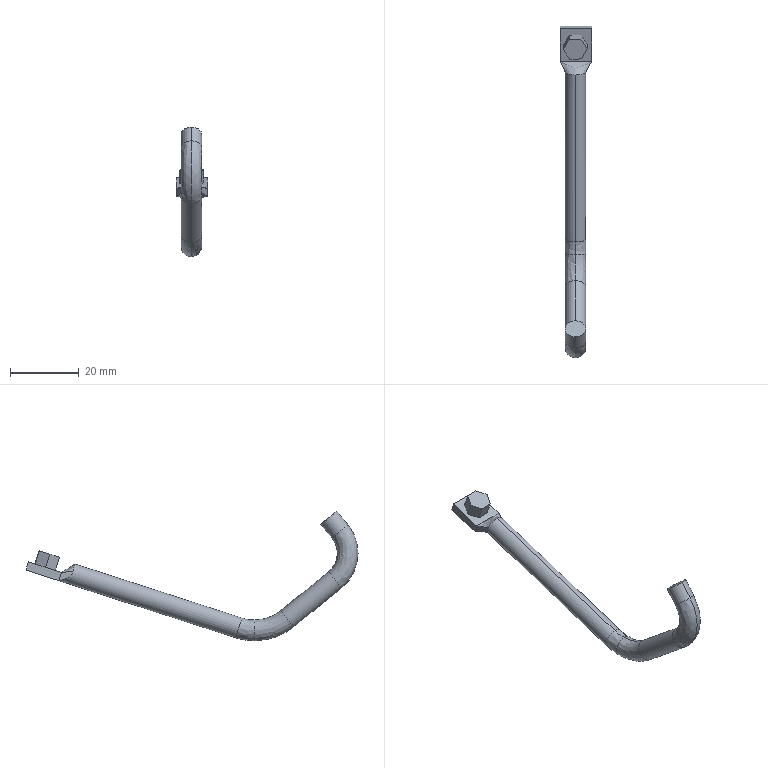Part | SolidWorks | features BaseBody 2 | 2 solids | 30 faces | box 9.082 x 96.3 x 37.547 mm | volume 3383 mm3 | plane 14 | spline 10 | cylinder 6 | commonest cylinder face diameters 6 x6
STEP:
#1=CARTESIAN_POINT('',(0.000000001,-80.618,2441.417));
#2=VERTEX_POINT('',#1);
#3=CARTESIAN_POINT('',(0.000000001,-76.83,2446.069));
#4=VERTEX_POINT('',#3);
#5=CARTESIAN_POINT('',(0.,-78.724,2443.743));
#6=DIRECTION('',(0.,-0.7755,0.6314));
#7=DIRECTION('',(0.,0.6314,0.7755));
#8=AXIS2_PLACEMENT_3D('',#5,#6,#7);
#9=CIRCLE('',#8,3.);
#10=EDGE_CURVE('',#2,#4,#9,.T.);
#11=ORIENTED_EDGE('',*,*,#10,.F.);
#12=CARTESIAN_POINT('',(0.,-66.764,2430.136));
#13=VERTEX_POINT('',#12);
#14=CARTESIAN_POINT('',(0.,-80.618,2441.417));
#15=DIRECTION('',(0.,0.7755,-0.6314));
#16=VECTOR('',#15,1000.);
#17=LINE('',#14,#16);
#18=EDGE_CURVE('',#2,#13,#17,.T.);
#19=ORIENTED_EDGE('',*,*,#18,.T.);
#20=CARTESIAN_POINT('',(0.000000001,-62.975,2434.789));
#21=VERTEX_POINT('',#20);
#22=CARTESIAN_POINT('',(0.,-64.869,2432.462));
#23=DIRECTION('',(0.,0.7755,-0.6314));
#24=DIRECTION('',(0.,0.6314,0.7755));
#25=AXIS2_PLACEMENT_3D('',#22,#23,#24);
#26=CIRCLE('',#25,3.);
#27=EDGE_CURVE('',#21,#13,#26,.T.);
#28=ORIENTED_EDGE('',*,*,#27,.F.);
#29=CARTESIAN_POINT('',(0.,-76.83,2446.069));
#30=DIRECTION('',(0.,0.7755,-0.6314));
#31=VECTOR('',#30,1000.);
#32=LINE('',#29,#31);
#33=EDGE_CURVE('',#4,#21,#32,.T.);
#34=ORIENTED_EDGE('',*,*,#33,.F.);
#35=EDGE_LOOP('',(#11,#19,#28,#34));
#36=FACE_OUTER_BOUND('',#35,.T.);
#37=CARTESIAN_POINT('',(0.,-78.724,2443.743));
#38=DIRECTION('',(0.,0.7755,-0.6314));
#39=DIRECTION('',(0.,0.6314,0.7755));
#40=AXIS2_PLACEMENT_3D('',#37,#38,#39);
#41=CYLINDRICAL_SURFACE('',#40,3.);
#42=ADVANCED_FACE('',(#36),#41,.T.);
#43=CARTESIAN_POINT('',(0.000000001,-77.838,2455.917));
#44=VERTEX_POINT('',#43);
#45=CARTESIAN_POINT('',(0.000000001,-82.491,2459.706));
#46=VERTEX_POINT('',#45);
#47=CARTESIAN_POINT('',(0.,-80.164,2457.811));
#48=DIRECTION('',(0.,-0.6314,-0.7755));
#49=DIRECTION('',(0.,-0.7755,0.6314));
#50=AXIS2_PLACEMENT_3D('',#47,#48,#49);
#51=CIRCLE('',#50,3.);
#52=EDGE_CURVE('',#44,#46,#51,.T.);
#53=ORIENTED_EDGE('',*,*,#52,.F.);
#54=CARTESIAN_POINT('',(0.,-74.634,2459.853));
#55=VERTEX_POINT('',#54);
#56=CARTESIAN_POINT('',(0.,-77.838,2455.917));
#57=DIRECTION('',(0.,0.6314,0.7755));
#58=VECTOR('',#57,1000.);
#59=LINE('',#56,#58);
#60=EDGE_CURVE('',#44,#55,#59,.T.);
#61=ORIENTED_EDGE('',*,*,#60,.T.);
#62=CARTESIAN_POINT('',(0.,-79.286,2463.641));
#63=VERTEX_POINT('',#62);
#64=CARTESIAN_POINT('',(0.,-76.96,2461.747));
#65=DIRECTION('',(0.,0.6314,0.7755));
#66=DIRECTION('',(0.,-0.7755,0.6314));
#67=AXIS2_PLACEMENT_3D('',#64,#65,#66);
#68=CIRCLE('',#67,3.);
#69=EDGE_CURVE('',#63,#55,#68,.T.);
#70=ORIENTED_EDGE('',*,*,#69,.F.);
#71=CARTESIAN_POINT('',(0.,-82.491,2459.706));
#72=DIRECTION('',(0.,0.6314,0.7755));
#73=VECTOR('',#72,1000.);
#74=LINE('',#71,#73);
#75=EDGE_CURVE('',#46,#63,#74,.T.);
#76=ORIENTED_EDGE('',*,*,#75,.F.);
#77=EDGE_LOOP('',(#53,#61,#70,#76));
#78=FACE_OUTER_BOUND('',#77,.T.);
#79=CARTESIAN_POINT('',(0.,-80.164,2457.811));
#80=DIRECTION('',(0.,0.6314,0.7755));
#81=DIRECTION('',(0.,-0.7755,0.6314));
#82=AXIS2_PLACEMENT_3D('',#79,#80,#81);
#83=CYLINDRICAL_SURFACE('',#82,3.);
#84=ADVANCED_FACE('',(#78),#83,.T.);
#85=CARTESIAN_POINT('',(0.000000001,-49.867,2426.965));
#86=VERTEX_POINT('',#85);
#87=CARTESIAN_POINT('',(0.000000001,-51.711,2432.675));
#88=VERTEX_POINT('',#87);
#89=CARTESIAN_POINT('',(0.,-50.789,2429.82));
#90=DIRECTION('',(0.,-0.9516,-0.3073));
#91=DIRECTION('',(0.,-0.3073,0.9516));
#92=AXIS2_PLACEMENT_3D('',#89,#90,#91);
#93=CIRCLE('',#92,3.);
#94=EDGE_CURVE('',#86,#88,#93,.T.);
#95=ORIENTED_EDGE('',*,*,#94,.F.);
#96=CARTESIAN_POINT('',(-0.000000001,-1.479,2442.591));
#97=VERTEX_POINT('',#96);
#98=CARTESIAN_POINT('',(0.,-49.867,2426.965));
#99=DIRECTION('',(0.,0.9516,0.3073));
#100=VECTOR('',#99,1000.);
#101=LINE('',#98,#100);
#102=EDGE_CURVE('',#86,#97,#101,.T.);
#103=ORIENTED_EDGE('',*,*,#102,.T.);
#104=CARTESIAN_POINT('',(2.892,-2.157,2444.688));
#105=VERTEX_POINT('',#104);
#106=CARTESIAN_POINT('',(2.892,-2.157,2444.688));
#107=CARTESIAN_POINT('',(2.828,-2.085,2444.467));
#108=CARTESIAN_POINT('',(2.73,-2.009,2444.232));
#109=CARTESIAN_POINT('',(2.439,-1.857,2443.761));
#110=CARTESIAN_POINT('',(2.244,-1.781,2443.525));
#111=CARTESIAN_POINT('',(1.748,-1.645,2443.104));
#112=CARTESIAN_POINT('',(1.445,-1.585,2442.919));
#113=CARTESIAN_POINT('',(0.761,-1.502,2442.662));
#114=CARTESIAN_POINT('',(0.381,-1.479,2442.591));
#115=CARTESIAN_POINT('',(-0.000000001,-1.479,2442.591));
#116=B_SPLINE_CURVE_WITH_KNOTS('',3,(#106,#107,#108,#109,#110,#111,#112,#113,#114,#115),.UNSPECIFIED.,.F.,.F.,(4,2,2,2,4),(0.,0.25,0.5,0.75,1.),.UNSPECIFIED.);
#117=EDGE_CURVE('',#105,#97,#116,.T.);
#118=ORIENTED_EDGE('',*,*,#117,.F.);
#119=CARTESIAN_POINT('',(2.892,-2.646,2446.203));
#120=VERTEX_POINT('',#119);
#121=CARTESIAN_POINT('',(2.892,-2.646,2446.203));
#122=CARTESIAN_POINT('',(2.963,-2.567,2445.96));
#123=CARTESIAN_POINT('',(3.,-2.484,2445.703));
#124=CARTESIAN_POINT('',(3.,-2.318,2445.189));
#125=CARTESIAN_POINT('',(2.963,-2.235,2444.932));
#126=CARTESIAN_POINT('',(2.892,-2.157,2444.688));
#127=B_SPLINE_CURVE_WITH_KNOTS('',3,(#121,#122,#123,#124,#125,#126),.UNSPECIFIED.,.F.,.F.,(4,2,4),(0.,0.5,1.),.UNSPECIFIED.);
#128=EDGE_CURVE('',#120,#105,#127,.T.);
#129=ORIENTED_EDGE('',*,*,#128,.F.);
#130=CARTESIAN_POINT('',(0.,-3.323,2448.301));
#131=VERTEX_POINT('',#130);
#132=CARTESIAN_POINT('',(0.,-3.323,2448.301));
#133=CARTESIAN_POINT('',(0.381,-3.323,2448.301));
#134=CARTESIAN_POINT('',(0.761,-3.3,2448.229));
#135=CARTESIAN_POINT('',(1.445,-3.217,2447.972));
#136=CARTESIAN_POINT('',(1.748,-3.158,2447.788));
#137=CARTESIAN_POINT('',(2.244,-3.021,2447.366));
#138=CARTESIAN_POINT('',(2.439,-2.945,2447.131));
#139=CARTESIAN_POINT('',(2.73,-2.793,2446.66));
#140=CARTESIAN_POINT('',(2.828,-2.717,2446.425));
#141=CARTESIAN_POINT('',(2.892,-2.646,2446.203));
#142=B_SPLINE_CURVE_WITH_KNOTS('',3,(#132,#133,#134,#135,#136,#137,#138,#139,#140,#141),.UNSPECIFIED.,.F.,.F.,(4,2,2,2,4),(0.,0.25,0.5,0.75,1.),.UNSPECIFIED.);
#143=EDGE_CURVE('',#131,#120,#142,.T.);
#144=ORIENTED_EDGE('',*,*,#143,.F.);
#145=CARTESIAN_POINT('',(0.,-51.711,2432.675));
#146=DIRECTION('',(0.,0.9516,0.3073));
#147=VECTOR('',#146,1000.);
#148=LINE('',#145,#147);
#149=EDGE_CURVE('',#88,#131,#148,.T.);
#150=ORIENTED_EDGE('',*,*,#149,.F.);
#151=EDGE_LOOP('',(#95,#103,#118,#129,#144,#150));
#152=FACE_OUTER_BOUND('',#151,.T.);
#153=CARTESIAN_POINT('',(0.,-50.789,2429.82));
#154=DIRECTION('',(0.,0.9516,0.3073));
#155=DIRECTION('',(0.,-0.3073,0.9516));
#156=AXIS2_PLACEMENT_3D('',#153,#154,#155);
#157=CYLINDRICAL_SURFACE('',#156,3.);
#158=ADVANCED_FACE('',(#152),#157,.T.);
#159=ORIENTED_EDGE('',*,*,#10,.T.);
#160=CARTESIAN_POINT('',(0.000000003,-72.41,2451.497));
#161=DIRECTION('',(-1.,0.,0.));
#162=DIRECTION('',(0.,-1.,0.));
#163=AXIS2_PLACEMENT_3D('',#160,#161,#162);
#164=CIRCLE('',#163,7.);
#165=EDGE_CURVE('',#4,#44,#164,.T.);
#166=ORIENTED_EDGE('',*,*,#165,.T.);
#167=ORIENTED_EDGE('',*,*,#52,.T.);
#168=CARTESIAN_POINT('',(0.000000001,-82.491,2459.706));
#169=CARTESIAN_POINT('',(0.000000003,-87.299,2453.8));
#170=CARTESIAN_POINT('',(0.000000003,-86.523,2446.225));
#171=CARTESIAN_POINT('',(0.000000001,-80.618,2441.417));
#172=(BOUNDED_CURVE()B_SPLINE_CURVE(3,(#168,#169,#170,#171),.UNSPECIFIED.,.F.,.F.)B_SPLINE_CURVE_WITH_KNOTS((4,4),(0.,1.),.UNSPECIFIED.)CURVE()GEOMETRIC_REPRESENTATION_ITEM()RATIONAL_B_SPLINE_CURVE((0.9594,0.7721,0.7721,0.9594))REPRESENTATION_ITEM(''));
#173=EDGE_CURVE('',#46,#2,#172,.T.);
#174=ORIENTED_EDGE('',*,*,#173,.T.);
#175=EDGE_LOOP('',(#159,#166,#167,#174));
#176=FACE_OUTER_BOUND('',#175,.T.);
#177=CARTESIAN_POINT('',(-0.2995,-77.85,2455.927));
#178=CARTESIAN_POINT('',(-0.2995,-80.444,2452.74));
#179=CARTESIAN_POINT('',(-0.2995,-80.026,2448.652));
#180=CARTESIAN_POINT('',(-0.2995,-76.839,2446.058));
#181=CARTESIAN_POINT('',(1.591,-77.702,2455.807));
#182=CARTESIAN_POINT('',(1.591,-80.227,2452.707));
#183=CARTESIAN_POINT('',(1.591,-79.82,2448.729));
#184=CARTESIAN_POINT('',(1.591,-76.719,2446.205));
#185=CARTESIAN_POINT('',(3.,-78.691,2456.612));
#186=CARTESIAN_POINT('',(3.,-81.687,2452.932));
#187=CARTESIAN_POINT('',(3.,-81.203,2448.212));
#188=CARTESIAN_POINT('',(3.,-77.524,2445.216));
#189=CARTESIAN_POINT('',(3.,-80.164,2457.811));
#190=CARTESIAN_POINT('',(3.,-83.863,2453.269));
#191=CARTESIAN_POINT('',(3.,-83.266,2447.442));
#192=CARTESIAN_POINT('',(3.,-78.724,2443.743));
#193=CARTESIAN_POINT('',(3.,-81.638,2459.011));
#194=CARTESIAN_POINT('',(3.,-86.039,2453.606));
#195=CARTESIAN_POINT('',(3.,-85.329,2446.671));
#196=CARTESIAN_POINT('',(3.,-79.923,2442.269));
#197=CARTESIAN_POINT('',(1.591,-82.626,2459.816));
#198=CARTESIAN_POINT('',(1.591,-87.499,2453.831));
#199=CARTESIAN_POINT('',(1.591,-86.713,2446.154));
#200=CARTESIAN_POINT('',(1.591,-80.728,2441.281));
#201=CARTESIAN_POINT('',(-0.2995,-82.479,2459.696));
#202=CARTESIAN_POINT('',(-0.2995,-87.282,2453.798));
#203=CARTESIAN_POINT('',(-0.2995,-86.507,2446.231));
#204=CARTESIAN_POINT('',(-0.2995,-80.608,2441.428));
#205=(BOUNDED_SURFACE()B_SPLINE_SURFACE(3,3,((#177,#178,#179,#180),(#181,#182,#183,#184),(#185,#186,#187,#188),(#189,#190,#191,#192),(#193,#194,#195,#196),(#197,#198,#199,#200),(#201,#202,#203,#204)),.UNSPECIFIED.,.F.,.F.,.T.)B_SPLINE_SURFACE_WITH_KNOTS((4,3,4),(4,4),(0.,0.5,1.),(0.,1.),.UNSPECIFIED.)GEOMETRIC_REPRESENTATION_ITEM()RATIONAL_B_SPLINE_SURFACE(((1.,0.8047,0.8047,1.),(0.7806,0.6282,0.6282,0.7806),(0.7806,0.6282,0.6282,0.7806),(1.,0.8047,0.8047,1.),(0.7806,0.6282,0.6282,0.7806),(0.7806,0.6282,0.6282,0.7806),(1.,0.8047,0.8047,1.)))REPRESENTATION_ITEM('')SURFACE());
#206=ADVANCED_FACE('',(#176),#205,.T.);
#207=ORIENTED_EDGE('',*,*,#165,.F.);
#208=CARTESIAN_POINT('',(0.,-78.724,2443.743));
#209=DIRECTION('',(0.,-0.7755,0.6314));
#210=DIRECTION('',(0.,0.6314,0.7755));
#211=AXIS2_PLACEMENT_3D('',#208,#209,#210);
#212=CIRCLE('',#211,3.);
#213=EDGE_CURVE('',#4,#2,#212,.T.);
#214=ORIENTED_EDGE('',*,*,#213,.T.);
#215=ORIENTED_EDGE('',*,*,#173,.F.);
#216=CARTESIAN_POINT('',(0.,-80.164,2457.811));
#217=DIRECTION('',(0.,-0.6314,-0.7755));
#218=DIRECTION('',(0.,-0.7755,0.6314));
#219=AXIS2_PLACEMENT_3D('',#216,#217,#218);
#220=CIRCLE('',#219,3.);
#221=EDGE_CURVE('',#46,#44,#220,.T.);
#222=ORIENTED_EDGE('',*,*,#221,.T.);
#223=EDGE_LOOP('',(#207,#214,#215,#222));
#224=FACE_OUTER_BOUND('',#223,.T.);
#225=CARTESIAN_POINT('',(0.2995,-82.479,2459.696));
#226=CARTESIAN_POINT('',(0.2995,-87.282,2453.798));
#227=CARTESIAN_POINT('',(0.2995,-86.507,2446.231));
#228=CARTESIAN_POINT('',(0.2995,-80.608,2441.428));
#229=CARTESIAN_POINT('',(-1.591,-82.626,2459.816));
#230=CARTESIAN_POINT('',(-1.591,-87.499,2453.831));
#231=CARTESIAN_POINT('',(-1.591,-86.713,2446.154));
#232=CARTESIAN_POINT('',(-1.591,-80.728,2441.281));
#233=CARTESIAN_POINT('',(-3.,-81.638,2459.011));
#234=CARTESIAN_POINT('',(-3.,-86.039,2453.606));
#235=CARTESIAN_POINT('',(-3.,-85.329,2446.671));
#236=CARTESIAN_POINT('',(-3.,-79.923,2442.269));
#237=CARTESIAN_POINT('',(-3.,-80.164,2457.811));
#238=CARTESIAN_POINT('',(-3.,-83.863,2453.269));
#239=CARTESIAN_POINT('',(-3.,-83.266,2447.442));
#240=CARTESIAN_POINT('',(-3.,-78.724,2443.743));
#241=CARTESIAN_POINT('',(-3.,-78.691,2456.612));
#242=CARTESIAN_POINT('',(-3.,-81.687,2452.932));
#243=CARTESIAN_POINT('',(-3.,-81.203,2448.212));
#244=CARTESIAN_POINT('',(-3.,-77.524,2445.216));
#245=CARTESIAN_POINT('',(-1.591,-77.702,2455.807));
#246=CARTESIAN_POINT('',(-1.591,-80.227,2452.707));
#247=CARTESIAN_POINT('',(-1.591,-79.82,2448.729));
#248=CARTESIAN_POINT('',(-1.591,-76.719,2446.205));
#249=CARTESIAN_POINT('',(0.2995,-77.85,2455.927));
#250=CARTESIAN_POINT('',(0.2995,-80.444,2452.74));
#251=CARTESIAN_POINT('',(0.2995,-80.026,2448.652));
#252=CARTESIAN_POINT('',(0.2995,-76.839,2446.058));
#253=(BOUNDED_SURFACE()B_SPLINE_SURFACE(3,3,((#225,#226,#227,#228),(#229,#230,#231,#232),(#233,#234,#235,#236),(#237,#238,#239,#240),(#241,#242,#243,#244),(#245,#246,#247,#248),(#249,#250,#251,#252)),.UNSPECIFIED.,.F.,.F.,.F.)B_SPLINE_SURFACE_WITH_KNOTS((4,3,4),(4,4),(0.,0.5,1.),(0.,1.),.UNSPECIFIED.)GEOMETRIC_REPRESENTATION_ITEM()RATIONAL_B_SPLINE_SURFACE(((1.,0.8047,0.8047,1.),(0.7806,0.6282,0.6282,0.7806),(0.7806,0.6282,0.6282,0.7806),(1.,0.8047,0.8047,1.),(0.7806,0.6282,0.6282,0.7806),(0.7806,0.6282,0.6282,0.7806),(1.,0.8047,0.8047,1.)))REPRESENTATION_ITEM('')SURFACE());
#254=ADVANCED_FACE('',(#224),#253,.T.);
#255=ORIENTED_EDGE('',*,*,#18,.F.);
#256=ORIENTED_EDGE('',*,*,#213,.F.);
#257=ORIENTED_EDGE('',*,*,#33,.T.);
#258=CARTESIAN_POINT('',(0.,-64.869,2432.462));
#259=DIRECTION('',(0.,0.7755,-0.6314));
#260=DIRECTION('',(0.,0.6314,0.7755));
#261=AXIS2_PLACEMENT_3D('',#258,#259,#260);
#262=CIRCLE('',#261,3.);
#263=EDGE_CURVE('',#13,#21,#262,.T.);
#264=ORIENTED_EDGE('',*,*,#263,.F.);
#265=EDGE_LOOP('',(#255,#256,#257,#264));
#266=FACE_OUTER_BOUND('',#265,.T.);
#267=CARTESIAN_POINT('',(0.,-78.724,2443.743));
#268=DIRECTION('',(0.,0.7755,-0.6314));
#269=DIRECTION('',(0.,0.6314,0.7755));
#270=AXIS2_PLACEMENT_3D('',#267,#268,#269);
#271=CYLINDRICAL_SURFACE('',#270,3.);
#272=ADVANCED_FACE('',(#266),#271,.T.);
#273=ORIENTED_EDGE('',*,*,#60,.F.);
#274=ORIENTED_EDGE('',*,*,#221,.F.);
#275=ORIENTED_EDGE('',*,*,#75,.T.);
#276=CARTESIAN_POINT('',(0.,-76.96,2461.747));
#277=DIRECTION('',(0.,0.6314,0.7755));
#278=DIRECTION('',(0.,-0.7755,0.6314));
#279=AXIS2_PLACEMENT_3D('',#276,#277,#278);
#280=CIRCLE('',#279,3.);
#281=EDGE_CURVE('',#55,#63,#280,.T.);
#282=ORIENTED_EDGE('',*,*,#281,.F.);
#283=EDGE_LOOP('',(#273,#274,#275,#282));
#284=FACE_OUTER_BOUND('',#283,.T.);
#285=CARTESIAN_POINT('',(0.,-80.164,2457.811));
#286=DIRECTION('',(0.,0.6314,0.7755));
#287=DIRECTION('',(0.,-0.7755,0.6314));
#288=AXIS2_PLACEMENT_3D('',#285,#286,#287);
#289=CYLINDRICAL_SURFACE('',#288,3.);
#290=ADVANCED_FACE('',(#284),#289,.T.);
#291=CARTESIAN_POINT('',(0.000000002,-55.398,2426.094));
#292=VERTEX_POINT('',#291);
#293=CARTESIAN_POINT('',(0.000000003,-55.398,2432.094));
#294=VERTEX_POINT('',#293);
#295=CARTESIAN_POINT('',(0.000000002,-55.398,2426.094));
#296=CARTESIAN_POINT('',(1.772,-55.398,2426.094));
#297=CARTESIAN_POINT('',(3.,-55.398,2427.352));
#298=CARTESIAN_POINT('',(3.,-55.398,2429.094));
#299=CARTESIAN_POINT('',(3.,-55.398,2430.836));
#300=CARTESIAN_POINT('',(1.772,-55.398,2432.094));
#301=CARTESIAN_POINT('',(0.000000003,-55.398,2432.094));
#302=(BOUNDED_CURVE()B_SPLINE_CURVE(3,(#295,#296,#297,#298,#299,#300,#301),.UNSPECIFIED.,.F.,.F.)B_SPLINE_CURVE_WITH_KNOTS((4,3,4),(0.03301,0.5,0.967),.UNSPECIFIED.)CURVE()GEOMETRIC_REPRESENTATION_ITEM()RATIONAL_B_SPLINE_CURVE((0.9594,0.7815,0.7951,1.,0.7951,0.7815,0.9594))REPRESENTATION_ITEM(''));
#303=EDGE_CURVE('',#292,#294,#302,.T.);
#304=ORIENTED_EDGE('',*,*,#303,.T.);
#305=CARTESIAN_POINT('',(0.000000003,-55.398,2444.094));
#306=DIRECTION('',(-1.,0.,0.));
#307=DIRECTION('',(0.,0.,1.));
#308=AXIS2_PLACEMENT_3D('',#305,#306,#307);
#309=CIRCLE('',#308,12.);
#310=EDGE_CURVE('',#294,#21,#309,.T.);
#311=ORIENTED_EDGE('',*,*,#310,.T.);
#312=ORIENTED_EDGE('',*,*,#27,.T.);
#313=CARTESIAN_POINT('',(0.000000003,-55.398,2444.094));
#314=DIRECTION('',(1.,0.,0.));
#315=DIRECTION('',(0.,0.,-1.));
#316=AXIS2_PLACEMENT_3D('',#313,#314,#315);
#317=CIRCLE('',#316,18.);
#318=EDGE_CURVE('',#13,#292,#317,.T.);
#319=ORIENTED_EDGE('',*,*,#318,.T.);
#320=EDGE_LOOP('',(#304,#311,#312,#319));
#321=FACE_OUTER_BOUND('',#320,.T.);
#322=CARTESIAN_POINT('',(-0.2995,-62.985,2434.777));
#323=CARTESIAN_POINT('',(-0.2995,-60.82,2433.014));
#324=CARTESIAN_POINT('',(-0.2995,-58.19,2432.079));
#325=CARTESIAN_POINT('',(-0.2995,-55.398,2432.079));
#326=CARTESIAN_POINT('',(1.591,-62.865,2434.924));
#327=CARTESIAN_POINT('',(1.591,-60.734,2433.189));
#328=CARTESIAN_POINT('',(1.591,-58.146,2432.269));
#329=CARTESIAN_POINT('',(1.591,-55.398,2432.269));
#330=CARTESIAN_POINT('',(3.,-63.67,2433.936));
#331=CARTESIAN_POINT('',(3.,-61.31,2432.014));
#332=CARTESIAN_POINT('',(3.,-58.442,2430.994));
#333=CARTESIAN_POINT('',(3.,-55.398,2430.994));
#334=CARTESIAN_POINT('',(3.,-64.869,2432.462));
#335=CARTESIAN_POINT('',(3.,-62.167,2430.262));
#336=CARTESIAN_POINT('',(3.,-58.883,2429.094));
#337=CARTESIAN_POINT('',(3.,-55.398,2429.094));
#338=CARTESIAN_POINT('',(3.,-66.069,2430.989));
#339=CARTESIAN_POINT('',(3.,-63.024,2428.51));
#340=CARTESIAN_POINT('',(3.,-59.325,2427.194));
#341=CARTESIAN_POINT('',(3.,-55.398,2427.194));
#342=CARTESIAN_POINT('',(1.591,-66.874,2430.));
#343=CARTESIAN_POINT('',(1.591,-63.599,2427.334));
#344=CARTESIAN_POINT('',(1.591,-59.621,2425.919));
#345=CARTESIAN_POINT('',(1.591,-55.398,2425.919));
#346=CARTESIAN_POINT('',(-0.2995,-66.754,2430.147));
#347=CARTESIAN_POINT('',(-0.2995,-63.514,2427.509));
#348=CARTESIAN_POINT('',(-0.2995,-59.577,2426.109));
#349=CARTESIAN_POINT('',(-0.2995,-55.398,2426.109));
#350=(BOUNDED_SURFACE()B_SPLINE_SURFACE(3,3,((#322,#323,#324,#325),(#326,#327,#328,#329),(#330,#331,#332,#333),(#334,#335,#336,#337),(#338,#339,#340,#341),(#342,#343,#344,#345),(#346,#347,#348,#349)),.UNSPECIFIED.,.F.,.F.,.T.)B_SPLINE_SURFACE_WITH_KNOTS((4,3,4),(4,4),(0.,0.5,1.),(0.,1.),.UNSPECIFIED.)GEOMETRIC_REPRESENTATION_ITEM()RATIONAL_B_SPLINE_SURFACE(((1.,0.9615,0.9615,1.),(0.7806,0.7505,0.7505,0.7806),(0.7806,0.7505,0.7505,0.7806),(1.,0.9615,0.9615,1.),(0.7806,0.7505,0.7505,0.7806),(0.7806,0.7505,0.7505,0.7806),(1.,0.9615,0.9615,1.)))REPRESENTATION_ITEM('')SURFACE());
#351=ADVANCED_FACE('',(#321),#350,.T.);
#352=ORIENTED_EDGE('',*,*,#69,.T.);
#353=ORIENTED_EDGE('',*,*,#281,.T.);
#354=EDGE_LOOP('',(#352,#353));
#355=FACE_OUTER_BOUND('',#354,.T.);
#356=CARTESIAN_POINT('',(-3.036,-74.606,2459.83));
#357=DIRECTION('',(0.,0.6314,0.7755));
#358=DIRECTION('',(0.,-0.7755,0.6314));
#359=AXIS2_PLACEMENT_3D('',#356,#357,#358);
#360=PLANE('',#359);
#361=ADVANCED_FACE('',(#355),#360,.T.);
#362=ORIENTED_EDGE('',*,*,#310,.F.);
#363=CARTESIAN_POINT('',(0.000000003,-55.398,2432.094));
#364=CARTESIAN_POINT('',(-1.772,-55.398,2432.094));
#365=CARTESIAN_POINT('',(-3.,-55.398,2430.836));
#366=CARTESIAN_POINT('',(-3.,-55.398,2429.094));
#367=CARTESIAN_POINT('',(-3.,-55.398,2427.352));
#368=CARTESIAN_POINT('',(-1.772,-55.398,2426.094));
#369=CARTESIAN_POINT('',(0.000000002,-55.398,2426.094));
#370=(BOUNDED_CURVE()B_SPLINE_CURVE(3,(#363,#364,#365,#366,#367,#368,#369),.UNSPECIFIED.,.F.,.F.)B_SPLINE_CURVE_WITH_KNOTS((4,3,4),(0.03301,0.5,0.967),.UNSPECIFIED.)CURVE()GEOMETRIC_REPRESENTATION_ITEM()RATIONAL_B_SPLINE_CURVE((0.9594,0.7815,0.7951,1.,0.7951,0.7815,0.9594))REPRESENTATION_ITEM(''));
#371=EDGE_CURVE('',#294,#292,#370,.T.);
#372=ORIENTED_EDGE('',*,*,#371,.T.);
#373=ORIENTED_EDGE('',*,*,#318,.F.);
#374=ORIENTED_EDGE('',*,*,#263,.T.);
#375=EDGE_LOOP('',(#362,#372,#373,#374));
#376=FACE_OUTER_BOUND('',#375,.T.);
#377=CARTESIAN_POINT('',(0.2995,-66.754,2430.147));
#378=CARTESIAN_POINT('',(0.2995,-63.514,2427.509));
#379=CARTESIAN_POINT('',(0.2995,-59.577,2426.109));
#380=CARTESIAN_POINT('',(0.2995,-55.398,2426.109));
#381=CARTESIAN_POINT('',(-1.591,-66.874,2430.));
#382=CARTESIAN_POINT('',(-1.591,-63.599,2427.334));
#383=CARTESIAN_POINT('',(-1.591,-59.621,2425.919));
#384=CARTESIAN_POINT('',(-1.591,-55.398,2425.919));
#385=CARTESIAN_POINT('',(-3.,-66.069,2430.989));
#386=CARTESIAN_POINT('',(-3.,-63.024,2428.51));
#387=CARTESIAN_POINT('',(-3.,-59.325,2427.194));
#388=CARTESIAN_POINT('',(-3.,-55.398,2427.194));
#389=CARTESIAN_POINT('',(-3.,-64.869,2432.462));
#390=CARTESIAN_POINT('',(-3.,-62.167,2430.262));
#391=CARTESIAN_POINT('',(-3.,-58.883,2429.094));
#392=CARTESIAN_POINT('',(-3.,-55.398,2429.094));
#393=CARTESIAN_POINT('',(-3.,-63.67,2433.936));
#394=CARTESIAN_POINT('',(-3.,-61.31,2432.014));
#395=CARTESIAN_POINT('',(-3.,-58.442,2430.994));
#396=CARTESIAN_POINT('',(-3.,-55.398,2430.994));
#397=CARTESIAN_POINT('',(-1.591,-62.865,2434.924));
#398=CARTESIAN_POINT('',(-1.591,-60.734,2433.189));
#399=CARTESIAN_POINT('',(-1.591,-58.146,2432.269));
#400=CARTESIAN_POINT('',(-1.591,-55.398,2432.269));
#401=CARTESIAN_POINT('',(0.2995,-62.985,2434.777));
#402=CARTESIAN_POINT('',(0.2995,-60.82,2433.014));
#403=CARTESIAN_POINT('',(0.2995,-58.19,2432.079));
#404=CARTESIAN_POINT('',(0.2995,-55.398,2432.079));
#405=(BOUNDED_SURFACE()B_SPLINE_SURFACE(3,3,((#377,#378,#379,#380),(#381,#382,#383,#384),(#385,#386,#387,#388),(#389,#390,#391,#392),(#393,#394,#395,#396),(#397,#398,#399,#400),(#401,#402,#403,#404)),.UNSPECIFIED.,.F.,.F.,.F.)B_SPLINE_SURFACE_WITH_KNOTS((4,3,4),(4,4),(0.,0.5,1.),(0.,1.),.UNSPECIFIED.)GEOMETRIC_REPRESENTATION_ITEM()RATIONAL_B_SPLINE_SURFACE(((1.,0.9615,0.9615,1.),(0.7806,0.7505,0.7505,0.7806),(0.7806,0.7505,0.7505,0.7806),(1.,0.9615,0.9615,1.),(0.7806,0.7505,0.7505,0.7806),(0.7806,0.7505,0.7505,0.7806),(1.,0.9615,0.9615,1.)))REPRESENTATION_ITEM('')SURFACE());
#406=ADVANCED_FACE('',(#376),#405,.T.);
#407=ORIENTED_EDGE('',*,*,#94,.T.);
#408=CARTESIAN_POINT('',(0.000000003,-55.398,2444.094));
#409=DIRECTION('',(-1.,0.,0.));
#410=DIRECTION('',(0.,0.,1.));
#411=AXIS2_PLACEMENT_3D('',#408,#409,#410);
#412=CIRCLE('',#411,12.);
#413=EDGE_CURVE('',#88,#294,#412,.T.);
#414=ORIENTED_EDGE('',*,*,#413,.T.);
#415=ORIENTED_EDGE('',*,*,#303,.F.);
#416=CARTESIAN_POINT('',(0.000000002,-55.398,2426.094));
#417=CARTESIAN_POINT('',(0.000000003,-53.517,2426.094));
#418=CARTESIAN_POINT('',(0.000000003,-51.658,2426.387));
#419=CARTESIAN_POINT('',(0.000000001,-49.867,2426.965));
#420=(BOUNDED_CURVE()B_SPLINE_CURVE(3,(#416,#417,#418,#419),.UNSPECIFIED.,.F.,.F.)B_SPLINE_CURVE_WITH_KNOTS((4,4),(0.,1.),.UNSPECIFIED.)CURVE()GEOMETRIC_REPRESENTATION_ITEM()RATIONAL_B_SPLINE_CURVE((0.9594,0.9516,0.9516,0.9594))REPRESENTATION_ITEM(''));
#421=EDGE_CURVE('',#292,#86,#420,.T.);
#422=ORIENTED_EDGE('',*,*,#421,.T.);
#423=EDGE_LOOP('',(#407,#414,#415,#422));
#424=FACE_OUTER_BOUND('',#423,.T.);
#425=CARTESIAN_POINT('',(-0.2995,-55.398,2432.079));
#426=CARTESIAN_POINT('',(-0.2995,-54.142,2432.079));
#427=CARTESIAN_POINT('',(-0.2995,-52.901,2432.274));
#428=CARTESIAN_POINT('',(-0.2995,-51.706,2432.66));
#429=CARTESIAN_POINT('',(1.591,-55.398,2432.269));
#430=CARTESIAN_POINT('',(1.591,-54.162,2432.269));
#431=CARTESIAN_POINT('',(1.591,-52.941,2432.461));
#432=CARTESIAN_POINT('',(1.591,-51.764,2432.841));
#433=CARTESIAN_POINT('',(3.,-55.398,2430.994));
#434=CARTESIAN_POINT('',(3.,-54.029,2430.994));
#435=CARTESIAN_POINT('',(3.,-52.676,2431.207));
#436=CARTESIAN_POINT('',(3.,-51.373,2431.628));
#437=CARTESIAN_POINT('',(3.,-55.398,2429.094));
#438=CARTESIAN_POINT('',(3.,-53.83,2429.094));
#439=CARTESIAN_POINT('',(3.,-52.281,2429.338));
#440=CARTESIAN_POINT('',(3.,-50.789,2429.82));
#441=CARTESIAN_POINT('',(3.,-55.398,2427.194));
#442=CARTESIAN_POINT('',(3.,-53.632,2427.194));
#443=CARTESIAN_POINT('',(3.,-51.886,2427.469));
#444=CARTESIAN_POINT('',(3.,-50.205,2428.012));
#445=CARTESIAN_POINT('',(1.591,-55.398,2425.919));
#446=CARTESIAN_POINT('',(1.591,-53.498,2425.919));
#447=CARTESIAN_POINT('',(1.591,-51.621,2426.215));
#448=CARTESIAN_POINT('',(1.591,-49.813,2426.799));
#449=CARTESIAN_POINT('',(-0.2995,-55.398,2426.109));
#450=CARTESIAN_POINT('',(-0.2995,-53.518,2426.109));
#451=CARTESIAN_POINT('',(-0.2995,-51.661,2426.401));
#452=CARTESIAN_POINT('',(-0.2995,-49.871,2426.979));
#453=(BOUNDED_SURFACE()B_SPLINE_SURFACE(3,3,((#425,#426,#427,#428),(#429,#430,#431,#432),(#433,#434,#435,#436),(#437,#438,#439,#440),(#441,#442,#443,#444),(#445,#446,#447,#448),(#449,#450,#451,#452)),.UNSPECIFIED.,.F.,.F.,.F.)B_SPLINE_SURFACE_WITH_KNOTS((4,3,4),(4,4),(0.,0.5,1.),(0.,1.),.UNSPECIFIED.)GEOMETRIC_REPRESENTATION_ITEM()RATIONAL_B_SPLINE_SURFACE(((1.,0.9919,0.9919,1.),(0.7806,0.7743,0.7743,0.7806),(0.7806,0.7743,0.7743,0.7806),(1.,0.9919,0.9919,1.),(0.7806,0.7743,0.7743,0.7806),(0.7806,0.7743,0.7743,0.7806),(1.,0.9919,0.9919,1.)))REPRESENTATION_ITEM('')SURFACE());
#454=ADVANCED_FACE('',(#424),#453,.T.);
#455=ORIENTED_EDGE('',*,*,#413,.F.);
#456=CARTESIAN_POINT('',(0.,-50.789,2429.82));
#457=DIRECTION('',(0.,-0.9516,-0.3073));
#458=DIRECTION('',(0.,-0.3073,0.9516));
#459=AXIS2_PLACEMENT_3D('',#456,#457,#458);
#460=CIRCLE('',#459,3.);
#461=EDGE_CURVE('',#88,#86,#460,.T.);
#462=ORIENTED_EDGE('',*,*,#461,.T.);
#463=ORIENTED_EDGE('',*,*,#421,.F.);
#464=ORIENTED_EDGE('',*,*,#371,.F.);
#465=EDGE_LOOP('',(#455,#462,#463,#464));
#466=FACE_OUTER_BOUND('',#465,.T.);
#467=CARTESIAN_POINT('',(0.2995,-55.398,2426.109));
#468=CARTESIAN_POINT('',(0.2995,-53.518,2426.109));
#469=CARTESIAN_POINT('',(0.2995,-51.661,2426.401));
#470=CARTESIAN_POINT('',(0.2995,-49.871,2426.979));
#471=CARTESIAN_POINT('',(-1.591,-55.398,2425.919));
#472=CARTESIAN_POINT('',(-1.591,-53.498,2425.919));
#473=CARTESIAN_POINT('',(-1.591,-51.621,2426.215));
#474=CARTESIAN_POINT('',(-1.591,-49.813,2426.799));
#475=CARTESIAN_POINT('',(-3.,-55.398,2427.194));
#476=CARTESIAN_POINT('',(-3.,-53.632,2427.194));
#477=CARTESIAN_POINT('',(-3.,-51.886,2427.469));
#478=CARTESIAN_POINT('',(-3.,-50.205,2428.012));
#479=CARTESIAN_POINT('',(-3.,-55.398,2429.094));
#480=CARTESIAN_POINT('',(-3.,-53.83,2429.094));
#481=CARTESIAN_POINT('',(-3.,-52.281,2429.338));
#482=CARTESIAN_POINT('',(-3.,-50.789,2429.82));
#483=CARTESIAN_POINT('',(-3.,-55.398,2430.994));
#484=CARTESIAN_POINT('',(-3.,-54.029,2430.994));
#485=CARTESIAN_POINT('',(-3.,-52.676,2431.207));
#486=CARTESIAN_POINT('',(-3.,-51.373,2431.628));
#487=CARTESIAN_POINT('',(-1.591,-55.398,2432.269));
#488=CARTESIAN_POINT('',(-1.591,-54.162,2432.269));
#489=CARTESIAN_POINT('',(-1.591,-52.941,2432.461));
#490=CARTESIAN_POINT('',(-1.591,-51.764,2432.841));
#491=CARTESIAN_POINT('',(0.2995,-55.398,2432.079));
#492=CARTESIAN_POINT('',(0.2995,-54.142,2432.079));
#493=CARTESIAN_POINT('',(0.2995,-52.901,2432.274));
#494=CARTESIAN_POINT('',(0.2995,-51.706,2432.66));
#495=(BOUNDED_SURFACE()B_SPLINE_SURFACE(3,3,((#467,#468,#469,#470),(#471,#472,#473,#474),(#475,#476,#477,#478),(#479,#480,#481,#482),(#483,#484,#485,#486),(#487,#488,#489,#490),(#491,#492,#493,#494)),.UNSPECIFIED.,.F.,.F.,.F.)B_SPLINE_SURFACE_WITH_KNOTS((4,3,4),(4,4),(0.,0.5,1.),(0.,1.),.UNSPECIFIED.)GEOMETRIC_REPRESENTATION_ITEM()RATIONAL_B_SPLINE_SURFACE(((1.,0.9919,0.9919,1.),(0.7806,0.7743,0.7743,0.7806),(0.7806,0.7743,0.7743,0.7806),(1.,0.9919,0.9919,1.),(0.7806,0.7743,0.7743,0.7806),(0.7806,0.7743,0.7743,0.7806),(1.,0.9919,0.9919,1.)))REPRESENTATION_ITEM('')SURFACE());
#496=ADVANCED_FACE('',(#466),#495,.T.);
#497=ORIENTED_EDGE('',*,*,#102,.F.);
#498=ORIENTED_EDGE('',*,*,#461,.F.);
#499=ORIENTED_EDGE('',*,*,#149,.T.);
#500=CARTESIAN_POINT('',(-2.892,-2.646,2446.203));
#501=VERTEX_POINT('',#500);
#502=CARTESIAN_POINT('',(-2.892,-2.646,2446.203));
#503=CARTESIAN_POINT('',(-2.828,-2.717,2446.425));
#504=CARTESIAN_POINT('',(-2.73,-2.793,2446.66));
#505=CARTESIAN_POINT('',(-2.439,-2.945,2447.131));
#506=CARTESIAN_POINT('',(-2.244,-3.021,2447.366));
#507=CARTESIAN_POINT('',(-1.748,-3.158,2447.788));
#508=CARTESIAN_POINT('',(-1.445,-3.217,2447.972));
#509=CARTESIAN_POINT('',(-0.761,-3.3,2448.229));
#510=CARTESIAN_POINT('',(-0.381,-3.323,2448.301));
#511=CARTESIAN_POINT('',(0.,-3.323,2448.301));
#512=B_SPLINE_CURVE_WITH_KNOTS('',3,(#502,#503,#504,#505,#506,#507,#508,#509,#510,#511),.UNSPECIFIED.,.F.,.F.,(4,2,2,2,4),(0.,0.25,0.5,0.75,1.),.UNSPECIFIED.);
#513=EDGE_CURVE('',#501,#131,#512,.T.);
#514=ORIENTED_EDGE('',*,*,#513,.F.);
#515=CARTESIAN_POINT('',(-2.892,-2.157,2444.688));
#516=VERTEX_POINT('',#515);
#517=CARTESIAN_POINT('',(-2.892,-2.157,2444.688));
#518=CARTESIAN_POINT('',(-2.963,-2.235,2444.932));
#519=CARTESIAN_POINT('',(-3.,-2.318,2445.189));
#520=CARTESIAN_POINT('',(-3.,-2.484,2445.703));
#521=CARTESIAN_POINT('',(-2.963,-2.567,2445.96));
#522=CARTESIAN_POINT('',(-2.892,-2.646,2446.203));
#523=B_SPLINE_CURVE_WITH_KNOTS('',3,(#517,#518,#519,#520,#521,#522),.UNSPECIFIED.,.F.,.F.,(4,2,4),(0.,0.5,1.),.UNSPECIFIED.);
#524=EDGE_CURVE('',#516,#501,#523,.T.);
#525=ORIENTED_EDGE('',*,*,#524,.F.);
#526=CARTESIAN_POINT('',(-0.000000001,-1.479,2442.591));
#527=CARTESIAN_POINT('',(-0.381,-1.479,2442.591));
#528=CARTESIAN_POINT('',(-0.761,-1.502,2442.662));
#529=CARTESIAN_POINT('',(-1.445,-1.585,2442.919));
#530=CARTESIAN_POINT('',(-1.748,-1.645,2443.104));
#531=CARTESIAN_POINT('',(-2.244,-1.781,2443.525));
#532=CARTESIAN_POINT('',(-2.439,-1.857,2443.761));
#533=CARTESIAN_POINT('',(-2.73,-2.009,2444.232));
#534=CARTESIAN_POINT('',(-2.828,-2.085,2444.467));
#535=CARTESIAN_POINT('',(-2.892,-2.157,2444.688));
#536=B_SPLINE_CURVE_WITH_KNOTS('',3,(#526,#527,#528,#529,#530,#531,#532,#533,#534,#535),.UNSPECIFIED.,.F.,.F.,(4,2,2,2,4),(0.,0.25,0.5,0.75,1.),.UNSPECIFIED.);
#537=EDGE_CURVE('',#97,#516,#536,.T.);
#538=ORIENTED_EDGE('',*,*,#537,.F.);
#539=EDGE_LOOP('',(#497,#498,#499,#514,#525,#538));
#540=FACE_OUTER_BOUND('',#539,.T.);
#541=CARTESIAN_POINT('',(0.,-50.789,2429.82));
#542=DIRECTION('',(0.,0.9516,0.3073));
#543=DIRECTION('',(0.,-0.3073,0.9516));
#544=AXIS2_PLACEMENT_3D('',#541,#542,#543);
#545=CYLINDRICAL_SURFACE('',#544,3.);
#546=ADVANCED_FACE('',(#540),#545,.T.);
#547=ORIENTED_EDGE('',*,*,#537,.T.);
#548=CARTESIAN_POINT('',(-4.356,1.375,2443.515));
#549=VERTEX_POINT('',#548);
#550=CARTESIAN_POINT('',(-3.624,-0.391,2444.102));
#551=DIRECTION('',(-0.366,0.8832,-0.2933));
#552=VECTOR('',#551,1000.);
#553=LINE('',#550,#552);
#554=EDGE_CURVE('',#516,#549,#553,.T.);
#555=ORIENTED_EDGE('',*,*,#554,.T.);
#556=CARTESIAN_POINT('',(4.726,1.375,2443.515));
#557=VERTEX_POINT('',#556);
#558=CARTESIAN_POINT('',(0.1852,1.375,2443.515));
#559=DIRECTION('',(1.,0.,0.));
#560=VECTOR('',#559,1000.);
#561=LINE('',#558,#560);
#562=EDGE_CURVE('',#549,#557,#561,.T.);
#563=ORIENTED_EDGE('',*,*,#562,.T.);
#564=CARTESIAN_POINT('',(3.809,-0.391,2444.102));
#565=DIRECTION('',(-0.4421,-0.8513,0.2827));
#566=VECTOR('',#565,1000.);
#567=LINE('',#564,#566);
#568=EDGE_CURVE('',#557,#105,#567,.T.);
#569=ORIENTED_EDGE('',*,*,#568,.T.);
#570=ORIENTED_EDGE('',*,*,#117,.T.);
#571=EDGE_LOOP('',(#547,#555,#563,#569,#570));
#572=FACE_OUTER_BOUND('',#571,.T.);
#573=CARTESIAN_POINT('',(-4.356,1.375,2443.515));
#574=CARTESIAN_POINT('',(-2.892,-2.157,2444.688));
#575=CARTESIAN_POINT('',(-3.978,1.375,2443.515));
#576=CARTESIAN_POINT('',(-2.828,-2.085,2444.467));
#577=CARTESIAN_POINT('',(-3.599,1.375,2443.515));
#578=CARTESIAN_POINT('',(-2.73,-2.009,2444.232));
#579=CARTESIAN_POINT('',(-2.842,1.375,2443.515));
#580=CARTESIAN_POINT('',(-2.439,-1.857,2443.761));
#581=CARTESIAN_POINT('',(-2.464,1.375,2443.515));
#582=CARTESIAN_POINT('',(-2.244,-1.781,2443.525));
#583=CARTESIAN_POINT('',(-1.707,1.375,2443.515));
#584=CARTESIAN_POINT('',(-1.748,-1.645,2443.104));
#585=CARTESIAN_POINT('',(-1.329,1.375,2443.515));
#586=CARTESIAN_POINT('',(-1.445,-1.585,2442.919));
#587=CARTESIAN_POINT('',(-0.5717,1.375,2443.515));
#588=CARTESIAN_POINT('',(-0.761,-1.502,2442.662));
#589=CARTESIAN_POINT('',(-0.1933,1.375,2443.515));
#590=CARTESIAN_POINT('',(-0.381,-1.479,2442.591));
#591=CARTESIAN_POINT('',(0.5636,1.375,2443.515));
#592=CARTESIAN_POINT('',(0.381,-1.479,2442.591));
#593=CARTESIAN_POINT('',(0.942,1.375,2443.515));
#594=CARTESIAN_POINT('',(0.761,-1.502,2442.662));
#595=CARTESIAN_POINT('',(1.699,1.375,2443.515));
#596=CARTESIAN_POINT('',(1.445,-1.585,2442.919));
#597=CARTESIAN_POINT('',(2.077,1.375,2443.515));
#598=CARTESIAN_POINT('',(1.748,-1.645,2443.104));
#599=CARTESIAN_POINT('',(2.834,1.375,2443.515));
#600=CARTESIAN_POINT('',(2.244,-1.781,2443.525));
#601=CARTESIAN_POINT('',(3.213,1.375,2443.515));
#602=CARTESIAN_POINT('',(2.439,-1.857,2443.761));
#603=CARTESIAN_POINT('',(3.97,1.375,2443.515));
#604=CARTESIAN_POINT('',(2.73,-2.009,2444.232));
#605=CARTESIAN_POINT('',(4.348,1.375,2443.515));
#606=CARTESIAN_POINT('',(2.828,-2.085,2444.467));
#607=CARTESIAN_POINT('',(4.726,1.375,2443.515));
#608=CARTESIAN_POINT('',(2.892,-2.157,2444.688));
#609=B_SPLINE_SURFACE_WITH_KNOTS('',3,1,((#573,#574),(#575,#576),(#577,#578),(#579,#580),(#581,#582),(#583,#584),(#585,#586),(#587,#588),(#589,#590),(#591,#592),(#593,#594),(#595,#596),(#597,#598),(#599,#600),(#601,#602),(#603,#604),(#605,#606),(#607,#608)),.UNSPECIFIED.,.F.,.F.,.F.,(4,2,2,2,2,2,2,2,4),(2,2),(0.,0.125,0.25,0.375,0.5,0.625,0.75,0.875,1.),(0.,1.),.UNSPECIFIED.);
#610=ADVANCED_FACE('',(#572),#609,.T.);
#611=ORIENTED_EDGE('',*,*,#143,.T.);
#612=CARTESIAN_POINT('',(4.726,0.6064,2445.894));
#613=VERTEX_POINT('',#612);
#614=CARTESIAN_POINT('',(3.809,-1.02,2446.049));
#615=DIRECTION('',(0.4895,0.8681,-0.08247));
#616=VECTOR('',#615,1000.);
#617=LINE('',#614,#616);
#618=EDGE_CURVE('',#120,#613,#617,.T.);
#619=ORIENTED_EDGE('',*,*,#618,.T.);
#620=CARTESIAN_POINT('',(-4.356,0.6064,2445.894));
#621=VERTEX_POINT('',#620);
#622=CARTESIAN_POINT('',(0.1852,0.6064,2445.894));
#623=DIRECTION('',(-1.,0.,0.));
#624=VECTOR('',#623,1000.);
#625=LINE('',#622,#624);
#626=EDGE_CURVE('',#613,#621,#625,.T.);
#627=ORIENTED_EDGE('',*,*,#626,.T.);
#628=CARTESIAN_POINT('',(-3.624,-1.02,2446.049));
#629=DIRECTION('',(0.4088,-0.9085,0.08631));
#630=VECTOR('',#629,1000.);
#631=LINE('',#628,#630);
#632=EDGE_CURVE('',#621,#501,#631,.T.);
#633=ORIENTED_EDGE('',*,*,#632,.T.);
#634=ORIENTED_EDGE('',*,*,#513,.T.);
#635=EDGE_LOOP('',(#611,#619,#627,#633,#634));
#636=FACE_OUTER_BOUND('',#635,.T.);
#637=CARTESIAN_POINT('',(4.726,0.6064,2445.894));
#638=CARTESIAN_POINT('',(2.892,-2.646,2446.203));
#639=CARTESIAN_POINT('',(4.348,0.6064,2445.894));
#640=CARTESIAN_POINT('',(2.828,-2.717,2446.425));
#641=CARTESIAN_POINT('',(3.97,0.6064,2445.894));
#642=CARTESIAN_POINT('',(2.73,-2.793,2446.66));
#643=CARTESIAN_POINT('',(3.213,0.6064,2445.894));
#644=CARTESIAN_POINT('',(2.439,-2.945,2447.131));
#645=CARTESIAN_POINT('',(2.834,0.6064,2445.894));
#646=CARTESIAN_POINT('',(2.244,-3.021,2447.366));
#647=CARTESIAN_POINT('',(2.077,0.6064,2445.894));
#648=CARTESIAN_POINT('',(1.748,-3.158,2447.788));
#649=CARTESIAN_POINT('',(1.699,0.6064,2445.894));
#650=CARTESIAN_POINT('',(1.445,-3.217,2447.972));
#651=CARTESIAN_POINT('',(0.942,0.6064,2445.894));
#652=CARTESIAN_POINT('',(0.761,-3.3,2448.229));
#653=CARTESIAN_POINT('',(0.5636,0.6064,2445.894));
#654=CARTESIAN_POINT('',(0.381,-3.323,2448.301));
#655=CARTESIAN_POINT('',(-0.1933,0.6064,2445.894));
#656=CARTESIAN_POINT('',(-0.381,-3.323,2448.301));
#657=CARTESIAN_POINT('',(-0.5717,0.6064,2445.894));
#658=CARTESIAN_POINT('',(-0.761,-3.3,2448.229));
#659=CARTESIAN_POINT('',(-1.329,0.6064,2445.894));
#660=CARTESIAN_POINT('',(-1.445,-3.217,2447.972));
#661=CARTESIAN_POINT('',(-1.707,0.6064,2445.894));
#662=CARTESIAN_POINT('',(-1.748,-3.158,2447.788));
#663=CARTESIAN_POINT('',(-2.464,0.6064,2445.894));
#664=CARTESIAN_POINT('',(-2.244,-3.021,2447.366));
#665=CARTESIAN_POINT('',(-2.842,0.6064,2445.894));
#666=CARTESIAN_POINT('',(-2.439,-2.945,2447.131));
#667=CARTESIAN_POINT('',(-3.599,0.6064,2445.894));
#668=CARTESIAN_POINT('',(-2.73,-2.793,2446.66));
#669=CARTESIAN_POINT('',(-3.978,0.6064,2445.894));
#670=CARTESIAN_POINT('',(-2.828,-2.717,2446.425));
#671=CARTESIAN_POINT('',(-4.356,0.6064,2445.894));
#672=CARTESIAN_POINT('',(-2.892,-2.646,2446.203));
#673=B_SPLINE_SURFACE_WITH_KNOTS('',3,1,((#637,#638),(#639,#640),(#641,#642),(#643,#644),(#645,#646),(#647,#648),(#649,#650),(#651,#652),(#653,#654),(#655,#656),(#657,#658),(#659,#660),(#661,#662),(#663,#664),(#665,#666),(#667,#668),(#669,#670),(#671,#672)),.UNSPECIFIED.,.F.,.F.,.F.,(4,2,2,2,2,2,2,2,4),(2,2),(0.,0.125,0.25,0.375,0.5,0.625,0.75,0.875,1.),(0.,1.),.UNSPECIFIED.);
#674=ADVANCED_FACE('',(#636),#673,.T.);
#675=ORIENTED_EDGE('',*,*,#524,.T.);
#676=ORIENTED_EDGE('',*,*,#632,.F.);
#677=CARTESIAN_POINT('',(-4.356,0.9905,2444.705));
#678=DIRECTION('',(0.,0.3073,-0.9516));
#679=VECTOR('',#678,1000.);
#680=LINE('',#677,#679);
#681=EDGE_CURVE('',#621,#549,#680,.T.);
#682=ORIENTED_EDGE('',*,*,#681,.T.);
#683=ORIENTED_EDGE('',*,*,#554,.F.);
#684=EDGE_LOOP('',(#675,#676,#682,#683));
#685=FACE_OUTER_BOUND('',#684,.T.);
#686=CARTESIAN_POINT('',(-4.356,0.6064,2445.894));
#687=CARTESIAN_POINT('',(-2.892,-2.646,2446.203));
#688=CARTESIAN_POINT('',(-4.356,0.7344,2445.498));
#689=CARTESIAN_POINT('',(-2.963,-2.567,2445.96));
#690=CARTESIAN_POINT('',(-4.356,0.8625,2445.101));
#691=CARTESIAN_POINT('',(-3.,-2.484,2445.703));
#692=CARTESIAN_POINT('',(-4.356,1.119,2444.308));
#693=CARTESIAN_POINT('',(-3.,-2.318,2445.189));
#694=CARTESIAN_POINT('',(-4.356,1.247,2443.912));
#695=CARTESIAN_POINT('',(-2.963,-2.235,2444.932));
#696=CARTESIAN_POINT('',(-4.356,1.375,2443.515));
#697=CARTESIAN_POINT('',(-2.892,-2.157,2444.688));
#698=B_SPLINE_SURFACE_WITH_KNOTS('',3,1,((#686,#687),(#688,#689),(#690,#691),(#692,#693),(#694,#695),(#696,#697)),.UNSPECIFIED.,.F.,.F.,.F.,(4,2,4),(2,2),(0.,0.5,1.),(0.,1.),.UNSPECIFIED.);
#699=ADVANCED_FACE('',(#685),#698,.T.);
#700=ORIENTED_EDGE('',*,*,#128,.T.);
#701=ORIENTED_EDGE('',*,*,#568,.F.);
#702=CARTESIAN_POINT('',(4.726,0.9905,2444.705));
#703=DIRECTION('',(0.,-0.3073,0.9516));
#704=VECTOR('',#703,1000.);
#705=LINE('',#702,#704);
#706=EDGE_CURVE('',#557,#613,#705,.T.);
#707=ORIENTED_EDGE('',*,*,#706,.T.);
#708=ORIENTED_EDGE('',*,*,#618,.F.);
#709=EDGE_LOOP('',(#700,#701,#707,#708));
#710=FACE_OUTER_BOUND('',#709,.T.);
#711=CARTESIAN_POINT('',(4.726,1.375,2443.515));
#712=CARTESIAN_POINT('',(2.892,-2.157,2444.688));
#713=CARTESIAN_POINT('',(4.726,1.247,2443.912));
#714=CARTESIAN_POINT('',(2.963,-2.235,2444.932));
#715=CARTESIAN_POINT('',(4.726,1.119,2444.308));
#716=CARTESIAN_POINT('',(3.,-2.318,2445.189));
#717=CARTESIAN_POINT('',(4.726,0.8625,2445.101));
#718=CARTESIAN_POINT('',(3.,-2.484,2445.703));
#719=CARTESIAN_POINT('',(4.726,0.7344,2445.498));
#720=CARTESIAN_POINT('',(2.963,-2.567,2445.96));
#721=CARTESIAN_POINT('',(4.726,0.6064,2445.894));
#722=CARTESIAN_POINT('',(2.892,-2.646,2446.203));
#723=B_SPLINE_SURFACE_WITH_KNOTS('',3,1,((#711,#712),(#713,#714),(#715,#716),(#717,#718),(#719,#720),(#721,#722)),.UNSPECIFIED.,.F.,.F.,.F.,(4,2,4),(2,2),(0.,0.5,1.),(0.,1.),.UNSPECIFIED.);
#724=ADVANCED_FACE('',(#710),#723,.T.);
#725=CARTESIAN_POINT('',(-4.356,10.891,2446.588));
#726=VERTEX_POINT('',#725);
#727=CARTESIAN_POINT('',(-4.356,6.133,2445.052));
#728=DIRECTION('',(0.,-0.9516,-0.3073));
#729=VECTOR('',#728,1000.);
#730=LINE('',#727,#729);
#731=EDGE_CURVE('',#726,#549,#730,.T.);
#732=ORIENTED_EDGE('',*,*,#731,.F.);
#733=CARTESIAN_POINT('',(4.726,10.891,2446.588));
#734=VERTEX_POINT('',#733);
#735=CARTESIAN_POINT('',(0.1852,10.891,2446.588));
#736=DIRECTION('',(-1.,0.,0.));
#737=VECTOR('',#736,1000.);
#738=LINE('',#735,#737);
#739=EDGE_CURVE('',#734,#726,#738,.T.);
#740=ORIENTED_EDGE('',*,*,#739,.F.);
#741=CARTESIAN_POINT('',(4.726,6.133,2445.052));
#742=DIRECTION('',(0.,0.9516,0.3073));
#743=VECTOR('',#742,1000.);
#744=LINE('',#741,#743);
#745=EDGE_CURVE('',#557,#734,#744,.T.);
#746=ORIENTED_EDGE('',*,*,#745,.F.);
#747=ORIENTED_EDGE('',*,*,#562,.F.);
#748=EDGE_LOOP('',(#732,#740,#746,#747));
#749=FACE_OUTER_BOUND('',#748,.T.);
#750=CARTESIAN_POINT('',(-4.356,10.891,2446.588));
#751=DIRECTION('',(0.,-0.3073,0.9516));
#752=DIRECTION('',(0.,-0.9516,-0.3073));
#753=AXIS2_PLACEMENT_3D('',#750,#751,#752);
#754=PLANE('',#753);
#755=ADVANCED_FACE('',(#749),#754,.F.);
#756=CARTESIAN_POINT('',(4.726,10.122,2448.967));
#757=VERTEX_POINT('',#756);
#758=CARTESIAN_POINT('',(4.726,5.364,2447.431));
#759=DIRECTION('',(0.,-0.9516,-0.3073));
#760=VECTOR('',#759,1000.);
#761=LINE('',#758,#760);
#762=EDGE_CURVE('',#757,#613,#761,.T.);
#763=ORIENTED_EDGE('',*,*,#762,.F.);
#764=CARTESIAN_POINT('',(-4.356,10.122,2448.967));
#765=VERTEX_POINT('',#764);
#766=CARTESIAN_POINT('',(0.1852,10.122,2448.967));
#767=DIRECTION('',(1.,0.,0.));
#768=VECTOR('',#767,1000.);
#769=LINE('',#766,#768);
#770=EDGE_CURVE('',#765,#757,#769,.T.);
#771=ORIENTED_EDGE('',*,*,#770,.F.);
#772=CARTESIAN_POINT('',(-4.356,5.364,2447.431));
#773=DIRECTION('',(0.,0.9516,0.3073));
#774=VECTOR('',#773,1000.);
#775=LINE('',#772,#774);
#776=EDGE_CURVE('',#621,#765,#775,.T.);
#777=ORIENTED_EDGE('',*,*,#776,.F.);
#778=ORIENTED_EDGE('',*,*,#626,.F.);
#779=EDGE_LOOP('',(#763,#771,#777,#778));
#780=FACE_OUTER_BOUND('',#779,.T.);
#781=CARTESIAN_POINT('',(-4.356,0.6064,2445.894));
#782=DIRECTION('',(0.,0.3073,-0.9516));
#783=DIRECTION('',(0.,0.9516,0.3073));
#784=AXIS2_PLACEMENT_3D('',#781,#782,#783);
#785=PLANE('',#784);
#786=ADVANCED_FACE('',(#780),#785,.F.);
#787=ORIENTED_EDGE('',*,*,#776,.T.);
#788=CARTESIAN_POINT('',(-4.356,10.891,2446.588));
#789=CARTESIAN_POINT('',(-4.356,10.635,2447.381));
#790=CARTESIAN_POINT('',(-4.356,10.379,2448.174));
#791=CARTESIAN_POINT('',(-4.356,10.122,2448.967));
#792=B_SPLINE_CURVE_WITH_KNOTS('',3,(#788,#789,#790,#791),.UNSPECIFIED.,.F.,.F.,(4,4),(0.,1.),.UNSPECIFIED.);
#793=EDGE_CURVE('',#726,#765,#792,.T.);
#794=ORIENTED_EDGE('',*,*,#793,.F.);
#795=ORIENTED_EDGE('',*,*,#731,.T.);
#796=ORIENTED_EDGE('',*,*,#681,.F.);
#797=EDGE_LOOP('',(#787,#794,#795,#796));
#798=FACE_OUTER_BOUND('',#797,.T.);
#799=CARTESIAN_POINT('',(-4.356,0.5447,2449.));
#800=DIRECTION('',(1.,0.,0.));
#801=DIRECTION('',(0.,0.,-1.));
#802=AXIS2_PLACEMENT_3D('',#799,#800,#801);
#803=PLANE('',#802);
#804=ADVANCED_FACE('',(#798),#803,.F.);
#805=ORIENTED_EDGE('',*,*,#745,.T.);
#806=CARTESIAN_POINT('',(4.726,10.122,2448.967));
#807=CARTESIAN_POINT('',(4.726,10.379,2448.174));
#808=CARTESIAN_POINT('',(4.726,10.635,2447.381));
#809=CARTESIAN_POINT('',(4.726,10.891,2446.588));
#810=B_SPLINE_CURVE_WITH_KNOTS('',3,(#806,#807,#808,#809),.UNSPECIFIED.,.F.,.F.,(4,4),(0.,1.),.UNSPECIFIED.);
#811=EDGE_CURVE('',#757,#734,#810,.T.);
#812=ORIENTED_EDGE('',*,*,#811,.F.);
#813=ORIENTED_EDGE('',*,*,#762,.T.);
#814=ORIENTED_EDGE('',*,*,#706,.F.);
#815=EDGE_LOOP('',(#805,#812,#813,#814));
#816=FACE_OUTER_BOUND('',#815,.T.);
#817=CARTESIAN_POINT('',(4.726,0.5447,2443.483));
#818=DIRECTION('',(-1.,0.,0.));
#819=DIRECTION('',(0.,0.,1.));
#820=AXIS2_PLACEMENT_3D('',#817,#818,#819);
#821=PLANE('',#820);
#822=ADVANCED_FACE('',(#816),#821,.F.);
#823=ORIENTED_EDGE('',*,*,#770,.T.);
#824=ORIENTED_EDGE('',*,*,#811,.T.);
#825=ORIENTED_EDGE('',*,*,#739,.T.);
#826=ORIENTED_EDGE('',*,*,#793,.T.);
#827=EDGE_LOOP('',(#823,#824,#825,#826));
#828=FACE_OUTER_BOUND('',#827,.T.);
#829=CARTESIAN_POINT('',(-4.356,10.891,2446.588));
#830=DIRECTION('',(0.,0.9516,0.3073));
#831=DIRECTION('',(0.,-0.3073,0.9516));
#832=AXIS2_PLACEMENT_3D('',#829,#830,#831);
#833=PLANE('',#832);
#834=ADVANCED_FACE('',(#828),#833,.T.);
#835=CLOSED_SHELL('',(#42,#84,#158,#206,#254,#272,#290,#351,#361,#406,#454,#496,#546,#610,#674,#699,#724,#755,#786,#804,#822,#834));
#836=MANIFOLD_SOLID_BREP('',#835);
#837=CARTESIAN_POINT('',(-1.621,1.218,2450.295));
#838=VERTEX_POINT('',#837);
#839=CARTESIAN_POINT('',(-1.621,2.448,2446.489));
#840=VERTEX_POINT('',#839);
#841=CARTESIAN_POINT('',(-1.621,2.448,2446.489));
#842=DIRECTION('',(0.,0.3073,-0.9516));
#843=VECTOR('',#842,1000.);
#844=LINE('',#841,#843);
#845=EDGE_CURVE('',#838,#840,#844,.T.);
#846=ORIENTED_EDGE('',*,*,#845,.F.);
#847=CARTESIAN_POINT('',(-3.462,4.011,2451.197));
#848=VERTEX_POINT('',#847);
#849=CARTESIAN_POINT('',(-3.462,4.011,2451.197));
#850=DIRECTION('',(0.5315,-0.8061,-0.2603));
#851=VECTOR('',#850,1000.);
#852=LINE('',#849,#851);
#853=EDGE_CURVE('',#848,#838,#852,.T.);
#854=ORIENTED_EDGE('',*,*,#853,.F.);
#855=CARTESIAN_POINT('',(-3.462,5.24,2447.391));
#856=VERTEX_POINT('',#855);
#857=CARTESIAN_POINT('',(-3.462,5.24,2447.391));
#858=DIRECTION('',(0.,-0.3073,0.9516));
#859=VECTOR('',#858,1000.);
#860=LINE('',#857,#859);
#861=EDGE_CURVE('',#856,#848,#860,.T.);
#862=ORIENTED_EDGE('',*,*,#861,.F.);
#863=CARTESIAN_POINT('',(-1.621,2.448,2446.489));
#864=DIRECTION('',(-0.5315,0.8061,0.2603));
#865=VECTOR('',#864,1000.);
#866=LINE('',#863,#865);
#867=EDGE_CURVE('',#840,#856,#866,.T.);
#868=ORIENTED_EDGE('',*,*,#867,.F.);
#869=EDGE_LOOP('',(#846,#854,#862,#868));
#870=FACE_OUTER_BOUND('',#869,.T.);
#871=CARTESIAN_POINT('',(-1.062,1.521,2446.461));
#872=DIRECTION('',(0.8471,0.5057,0.1633));
#873=DIRECTION('',(-0.5126,0.8586,0.));
#874=AXIS2_PLACEMENT_3D('',#871,#872,#873);
#875=PLANE('',#874);
#876=ADVANCED_FACE('',(#870),#875,.F.);
#877=CARTESIAN_POINT('',(-1.841,8.153,2448.332));
#878=VERTEX_POINT('',#877);
#879=CARTESIAN_POINT('',(-1.841,8.153,2448.332));
#880=DIRECTION('',(-0.4679,-0.841,-0.2716));
#881=VECTOR('',#880,1000.);
#882=LINE('',#879,#881);
#883=EDGE_CURVE('',#878,#856,#882,.T.);
#884=ORIENTED_EDGE('',*,*,#883,.F.);
#885=CARTESIAN_POINT('',(1.621,8.275,2448.371));
#886=VERTEX_POINT('',#885);
#887=CARTESIAN_POINT('',(-1.841,8.153,2448.332));
#888=DIRECTION('',(-0.9993,-0.03494,-0.01128));
#889=VECTOR('',#888,1000.);
#890=LINE('',#887,#889);
#891=EDGE_CURVE('',#886,#878,#890,.T.);
#892=ORIENTED_EDGE('',*,*,#891,.F.);
#893=CARTESIAN_POINT('',(3.462,5.482,2447.469));
#894=VERTEX_POINT('',#893);
#895=CARTESIAN_POINT('',(3.462,5.482,2447.469));
#896=DIRECTION('',(-0.5315,0.8061,0.2603));
#897=VECTOR('',#896,1000.);
#898=LINE('',#895,#897);
#899=EDGE_CURVE('',#894,#886,#898,.T.);
#900=ORIENTED_EDGE('',*,*,#899,.F.);
#901=CARTESIAN_POINT('',(1.841,2.569,2446.528));
#902=VERTEX_POINT('',#901);
#903=CARTESIAN_POINT('',(1.841,2.569,2446.528));
#904=DIRECTION('',(0.4679,0.841,0.2716));
#905=VECTOR('',#904,1000.);
#906=LINE('',#903,#905);
#907=EDGE_CURVE('',#902,#894,#906,.T.);
#908=ORIENTED_EDGE('',*,*,#907,.F.);
#909=CARTESIAN_POINT('',(-1.621,2.448,2446.489));
#910=DIRECTION('',(0.9993,0.03494,0.01128));
#911=VECTOR('',#910,1000.);
#912=LINE('',#909,#911);
#913=EDGE_CURVE('',#840,#902,#912,.T.);
#914=ORIENTED_EDGE('',*,*,#913,.F.);
#915=ORIENTED_EDGE('',*,*,#867,.T.);
#916=EDGE_LOOP('',(#884,#892,#900,#908,#914,#915));
#917=FACE_OUTER_BOUND('',#916,.T.);
#918=CARTESIAN_POINT('',(-3.462,8.275,2448.371));
#919=DIRECTION('',(0.,-0.3073,0.9516));
#920=DIRECTION('',(0.,-0.9516,-0.3073));
#921=AXIS2_PLACEMENT_3D('',#918,#919,#920);
#922=PLANE('',#921);
#923=ADVANCED_FACE('',(#917),#922,.F.);
#924=CARTESIAN_POINT('',(1.841,1.339,2450.335));
#925=VERTEX_POINT('',#924);
#926=CARTESIAN_POINT('',(1.841,1.954,2448.431));
#927=DIRECTION('',(0.,0.3073,-0.9516));
#928=VECTOR('',#927,1000.);
#929=LINE('',#926,#928);
#930=EDGE_CURVE('',#925,#902,#929,.T.);
#931=ORIENTED_EDGE('',*,*,#930,.F.);
#932=CARTESIAN_POINT('',(0.1102,1.279,2450.315));
#933=DIRECTION('',(0.9993,0.03494,0.01128));
#934=VECTOR('',#933,1000.);
#935=LINE('',#932,#934);
#936=EDGE_CURVE('',#838,#925,#935,.T.);
#937=ORIENTED_EDGE('',*,*,#936,.F.);
#938=ORIENTED_EDGE('',*,*,#845,.T.);
#939=ORIENTED_EDGE('',*,*,#913,.T.);
#940=EDGE_LOOP('',(#931,#937,#938,#939));
#941=FACE_OUTER_BOUND('',#940,.T.);
#942=CARTESIAN_POINT('',(-1.621,2.448,2446.489));
#943=DIRECTION('',(-0.03672,0.951,0.3071));
#944=DIRECTION('',(0.,-0.3073,0.9516));
#945=AXIS2_PLACEMENT_3D('',#942,#943,#944);
#946=PLANE('',#945);
#947=ADVANCED_FACE('',(#941),#946,.F.);
#948=CARTESIAN_POINT('',(1.621,7.045,2452.177));
#949=VERTEX_POINT('',#948);
#950=CARTESIAN_POINT('',(-1.841,6.924,2452.138));
#951=VERTEX_POINT('',#950);
#952=CARTESIAN_POINT('',(1.621,7.045,2452.177));
#953=DIRECTION('',(-0.9993,-0.03494,-0.01128));
#954=VECTOR('',#953,1000.);
#955=LINE('',#952,#954);
#956=EDGE_CURVE('',#949,#951,#955,.T.);
#957=ORIENTED_EDGE('',*,*,#956,.T.);
#958=CARTESIAN_POINT('',(-1.841,6.924,2452.138));
#959=DIRECTION('',(-0.4679,-0.841,-0.2716));
#960=VECTOR('',#959,1000.);
#961=LINE('',#958,#960);
#962=EDGE_CURVE('',#951,#848,#961,.T.);
#963=ORIENTED_EDGE('',*,*,#962,.T.);
#964=ORIENTED_EDGE('',*,*,#853,.T.);
#965=ORIENTED_EDGE('',*,*,#936,.T.);
#966=CARTESIAN_POINT('',(3.462,4.253,2451.275));
#967=VERTEX_POINT('',#966);
#968=CARTESIAN_POINT('',(1.841,1.339,2450.335));
#969=DIRECTION('',(0.4679,0.841,0.2716));
#970=VECTOR('',#969,1000.);
#971=LINE('',#968,#970);
#972=EDGE_CURVE('',#925,#967,#971,.T.);
#973=ORIENTED_EDGE('',*,*,#972,.T.);
#974=CARTESIAN_POINT('',(3.462,4.253,2451.275));
#975=DIRECTION('',(-0.5315,0.8061,0.2603));
#976=VECTOR('',#975,1000.);
#977=LINE('',#974,#976);
#978=EDGE_CURVE('',#967,#949,#977,.T.);
#979=ORIENTED_EDGE('',*,*,#978,.T.);
#980=EDGE_LOOP('',(#957,#963,#964,#965,#973,#979));
#981=FACE_OUTER_BOUND('',#980,.T.);
#982=CARTESIAN_POINT('',(-3.462,7.045,2452.177));
#983=DIRECTION('',(0.,-0.3073,0.9516));
#984=DIRECTION('',(0.,-0.9516,-0.3073));
#985=AXIS2_PLACEMENT_3D('',#982,#983,#984);
#986=PLANE('',#985);
#987=ADVANCED_FACE('',(#981),#986,.T.);
#988=ORIENTED_EDGE('',*,*,#861,.T.);
#989=ORIENTED_EDGE('',*,*,#962,.F.);
#990=CARTESIAN_POINT('',(-1.841,6.924,2452.138));
#991=DIRECTION('',(0.,-0.3073,0.9516));
#992=VECTOR('',#991,1000.);
#993=LINE('',#990,#992);
#994=EDGE_CURVE('',#878,#951,#993,.T.);
#995=ORIENTED_EDGE('',*,*,#994,.F.);
#996=ORIENTED_EDGE('',*,*,#883,.T.);
#997=EDGE_LOOP('',(#988,#989,#995,#996));
#998=FACE_OUTER_BOUND('',#997,.T.);
#999=CARTESIAN_POINT('',(-3.971,4.238,2447.362));
#1000=DIRECTION('',(0.8838,-0.4452,-0.1438));
#1001=DIRECTION('',(0.4499,0.8931,0.));
#1002=AXIS2_PLACEMENT_3D('',#999,#1000,#1001);
#1003=PLANE('',#1002);
#1004=ADVANCED_FACE('',(#998),#1003,.F.);
#1005=ORIENTED_EDGE('',*,*,#994,.T.);
#1006=ORIENTED_EDGE('',*,*,#956,.F.);
#1007=CARTESIAN_POINT('',(1.621,7.66,2450.274));
#1008=DIRECTION('',(0.,-0.3073,0.9516));
#1009=VECTOR('',#1008,1000.);
#1010=LINE('',#1007,#1009);
#1011=EDGE_CURVE('',#886,#949,#1010,.T.);
#1012=ORIENTED_EDGE('',*,*,#1011,.F.);
#1013=ORIENTED_EDGE('',*,*,#891,.T.);
#1014=EDGE_LOOP('',(#1005,#1006,#1012,#1013));
#1015=FACE_OUTER_BOUND('',#1014,.T.);
#1016=CARTESIAN_POINT('',(-1.841,6.924,2452.138));
#1017=DIRECTION('',(0.03672,-0.951,-0.3071));
#1018=DIRECTION('',(0.,0.3073,-0.9516));
#1019=AXIS2_PLACEMENT_3D('',#1016,#1017,#1018);
#1020=PLANE('',#1019);
#1021=ADVANCED_FACE('',(#1015),#1020,.F.);
#1022=ORIENTED_EDGE('',*,*,#1011,.T.);
#1023=ORIENTED_EDGE('',*,*,#978,.F.);
#1024=CARTESIAN_POINT('',(3.462,5.482,2447.469));
#1025=DIRECTION('',(0.,-0.3073,0.9516));
#1026=VECTOR('',#1025,1000.);
#1027=LINE('',#1024,#1026);
#1028=EDGE_CURVE('',#894,#967,#1027,.T.);
#1029=ORIENTED_EDGE('',*,*,#1028,.F.);
#1030=ORIENTED_EDGE('',*,*,#899,.T.);
#1031=EDGE_LOOP('',(#1022,#1023,#1029,#1030));
#1032=FACE_OUTER_BOUND('',#1031,.T.);
#1033=CARTESIAN_POINT('',(1.739,8.376,2447.441));
#1034=DIRECTION('',(-0.8471,-0.5057,-0.1633));
#1035=DIRECTION('',(0.5126,-0.8586,0.));
#1036=AXIS2_PLACEMENT_3D('',#1033,#1034,#1035);
#1037=PLANE('',#1036);
#1038=ADVANCED_FACE('',(#1032),#1037,.F.);
#1039=ORIENTED_EDGE('',*,*,#1028,.T.);
#1040=ORIENTED_EDGE('',*,*,#972,.F.);
#1041=ORIENTED_EDGE('',*,*,#930,.T.);
#1042=ORIENTED_EDGE('',*,*,#907,.T.);
#1043=EDGE_LOOP('',(#1039,#1040,#1041,#1042));
#1044=FACE_OUTER_BOUND('',#1043,.T.);
#1045=CARTESIAN_POINT('',(3.348,5.569,2446.5));
#1046=DIRECTION('',(-0.8838,0.4452,0.1438));
#1047=DIRECTION('',(-0.4499,-0.8931,0.));
#1048=AXIS2_PLACEMENT_3D('',#1045,#1046,#1047);
#1049=PLANE('',#1048);
#1050=ADVANCED_FACE('',(#1044),#1049,.F.);
#1051=CLOSED_SHELL('',(#876,#923,#947,#987,#1004,#1021,#1038,#1050));
#1052=MANIFOLD_SOLID_BREP('',#1051);
#1053=CARTESIAN_POINT('',(0.,0.,0.));
#1054=DIRECTION('',(0.,0.,1.));
#1055=DIRECTION('',(1.,0.,0.));
#1056=AXIS2_PLACEMENT_3D('',#1053,#1054,#1055);
#1057=(LENGTH_UNIT()NAMED_UNIT(*)SI_UNIT(.MILLI.,.METRE.));
#1058=UNCERTAINTY_MEASURE_WITH_UNIT(LENGTH_MEASURE(0.00001),#1057,'','');
#1059=(NAMED_UNIT(*)PLANE_ANGLE_UNIT()SI_UNIT($,.RADIAN.));
#1060=(NAMED_UNIT(*)SI_UNIT($,.STERADIAN.)SOLID_ANGLE_UNIT());
#1061=(GEOMETRIC_REPRESENTATION_CONTEXT(3)GLOBAL_UNCERTAINTY_ASSIGNED_CONTEXT((#1058))GLOBAL_UNIT_ASSIGNED_CONTEXT((#1057,#1059,#1060))REPRESENTATION_CONTEXT('',''));
#1062=ADVANCED_BREP_SHAPE_REPRESENTATION('',(#836,#1052,#1056),#1061);